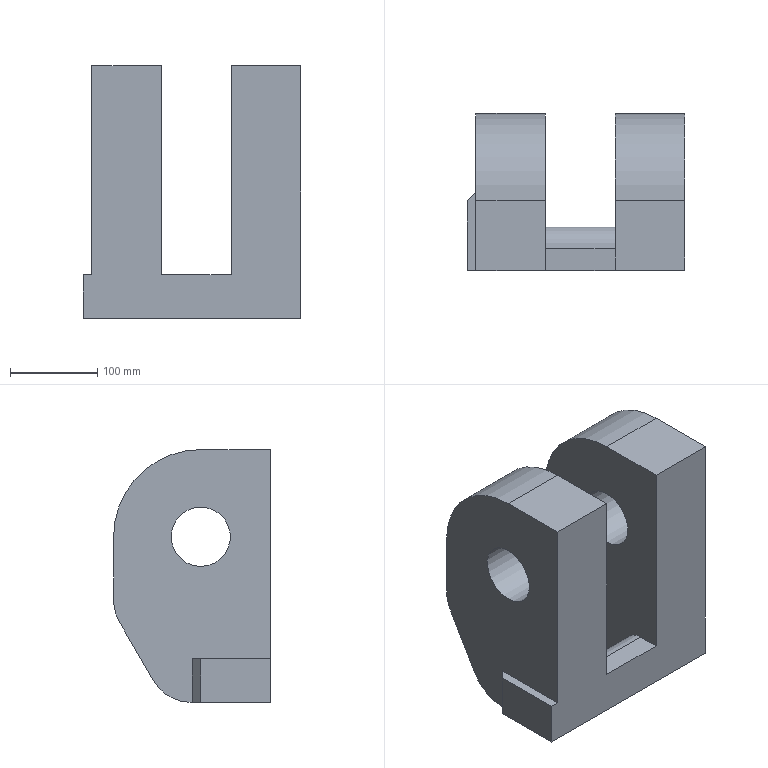Part | NX | features solid 2 | 1 solid | 25 faces | box 250 x 180 x 290 mm | volume 7125817 mm3 | plane 16 | cylinder 9 | commonest cylinder face diameters 100 x4 68 x2 200 x2 50 x1
STEP:
#1=CARTESIAN_POINT('',(-1345.,815.,-350.));
#2=VERTEX_POINT('',#1);
#3=CARTESIAN_POINT('',(-1425.,815.,-350.));
#4=VERTEX_POINT('',#3);
#5=CARTESIAN_POINT('',(-1345.,815.,-350.));
#6=DIRECTION('',(-1.,0.,0.));
#7=VECTOR('',#6,1000.);
#8=LINE('',#5,#7);
#9=EDGE_CURVE('',#2,#4,#8,.T.);
#10=ORIENTED_EDGE('',*,*,#9,.T.);
#11=CARTESIAN_POINT('',(-1425.,715.,-250.));
#12=VERTEX_POINT('',#11);
#13=CARTESIAN_POINT('',(-1425.,715.,-350.));
#14=DIRECTION('',(-1.,0.,0.));
#15=DIRECTION('',(0.,0.,-1.));
#16=AXIS2_PLACEMENT_3D('',#13,#14,#15);
#17=CIRCLE('',#16,100.);
#18=EDGE_CURVE('',#12,#4,#17,.T.);
#19=ORIENTED_EDGE('',*,*,#18,.F.);
#20=CARTESIAN_POINT('',(-1345.,715.,-250.));
#21=VERTEX_POINT('',#20);
#22=CARTESIAN_POINT('',(415.,715.,-250.));
#23=DIRECTION('',(1.,0.,0.));
#24=VECTOR('',#23,1000.);
#25=LINE('',#22,#24);
#26=EDGE_CURVE('',#21,#12,#25,.F.);
#27=ORIENTED_EDGE('',*,*,#26,.F.);
#28=CARTESIAN_POINT('',(-1345.,715.,-350.));
#29=DIRECTION('',(1.,0.,0.));
#30=DIRECTION('',(0.,0.,1.));
#31=AXIS2_PLACEMENT_3D('',#28,#29,#30);
#32=CIRCLE('',#31,100.);
#33=EDGE_CURVE('',#21,#2,#32,.F.);
#34=ORIENTED_EDGE('',*,*,#33,.T.);
#35=EDGE_LOOP('',(#10,#19,#27,#34));
#36=FACE_BOUND('',#35,.T.);
#37=CARTESIAN_POINT('',(415.,715.,-350.));
#38=DIRECTION('',(-1.,0.,0.));
#39=DIRECTION('',(0.,0.,1.));
#40=AXIS2_PLACEMENT_3D('',#37,#38,#39);
#41=CYLINDRICAL_SURFACE('',#40,100.);
#42=ADVANCED_FACE('',(#36),#41,.T.);
#43=CARTESIAN_POINT('',(-1505.,815.,-350.));
#44=VERTEX_POINT('',#43);
#45=CARTESIAN_POINT('',(-1585.,815.,-350.));
#46=VERTEX_POINT('',#45);
#47=CARTESIAN_POINT('',(-1505.,815.,-350.));
#48=DIRECTION('',(-1.,0.,0.));
#49=VECTOR('',#48,1000.);
#50=LINE('',#47,#49);
#51=EDGE_CURVE('',#44,#46,#50,.T.);
#52=ORIENTED_EDGE('',*,*,#51,.T.);
#53=CARTESIAN_POINT('',(-1585.,715.,-250.));
#54=VERTEX_POINT('',#53);
#55=CARTESIAN_POINT('',(-1585.,715.,-350.));
#56=DIRECTION('',(-1.,0.,0.));
#57=DIRECTION('',(0.,0.,-1.));
#58=AXIS2_PLACEMENT_3D('',#55,#56,#57);
#59=CIRCLE('',#58,100.);
#60=EDGE_CURVE('',#54,#46,#59,.T.);
#61=ORIENTED_EDGE('',*,*,#60,.F.);
#62=CARTESIAN_POINT('',(-1505.,715.,-250.));
#63=VERTEX_POINT('',#62);
#64=CARTESIAN_POINT('',(415.,715.,-250.));
#65=DIRECTION('',(1.,0.,0.));
#66=VECTOR('',#65,1000.);
#67=LINE('',#64,#66);
#68=EDGE_CURVE('',#63,#54,#67,.F.);
#69=ORIENTED_EDGE('',*,*,#68,.F.);
#70=CARTESIAN_POINT('',(-1505.,715.,-350.));
#71=DIRECTION('',(1.,0.,0.));
#72=DIRECTION('',(0.,0.,1.));
#73=AXIS2_PLACEMENT_3D('',#70,#71,#72);
#74=CIRCLE('',#73,100.);
#75=EDGE_CURVE('',#63,#44,#74,.F.);
#76=ORIENTED_EDGE('',*,*,#75,.T.);
#77=EDGE_LOOP('',(#52,#61,#69,#76));
#78=FACE_BOUND('',#77,.T.);
#79=CARTESIAN_POINT('',(415.,715.,-350.));
#80=DIRECTION('',(-1.,0.,0.));
#81=DIRECTION('',(0.,0.,1.));
#82=AXIS2_PLACEMENT_3D('',#79,#80,#81);
#83=CYLINDRICAL_SURFACE('',#82,100.);
#84=ADVANCED_FACE('',(#78),#83,.T.);
#85=CARTESIAN_POINT('',(-1345.,635.,-540.));
#86=VERTEX_POINT('',#85);
#87=CARTESIAN_POINT('',(-1345.,635.,-250.));
#88=VERTEX_POINT('',#87);
#89=CARTESIAN_POINT('',(-1345.,635.,-265.));
#90=DIRECTION('',(0.,0.,1.));
#91=VECTOR('',#90,1000.);
#92=LINE('',#89,#91);
#93=EDGE_CURVE('',#86,#88,#92,.T.);
#94=ORIENTED_EDGE('',*,*,#93,.T.);
#95=CARTESIAN_POINT('',(-1425.,635.,-250.));
#96=VERTEX_POINT('',#95);
#97=CARTESIAN_POINT('',(377.,635.,-250.));
#98=DIRECTION('',(-1.,0.,0.));
#99=VECTOR('',#98,1000.);
#100=LINE('',#97,#99);
#101=EDGE_CURVE('',#88,#96,#100,.T.);
#102=ORIENTED_EDGE('',*,*,#101,.T.);
#103=CARTESIAN_POINT('',(-1425.,635.,-490.));
#104=VERTEX_POINT('',#103);
#105=CARTESIAN_POINT('',(-1425.,635.,-350.));
#106=DIRECTION('',(0.,0.,1.));
#107=VECTOR('',#106,1000.);
#108=LINE('',#105,#107);
#109=EDGE_CURVE('',#104,#96,#108,.T.);
#110=ORIENTED_EDGE('',*,*,#109,.F.);
#111=CARTESIAN_POINT('',(-1505.,635.,-490.));
#112=VERTEX_POINT('',#111);
#113=CARTESIAN_POINT('',(1195.,635.,-490.));
#114=DIRECTION('',(-1.,0.,0.));
#115=VECTOR('',#114,1000.);
#116=LINE('',#113,#115);
#117=EDGE_CURVE('',#104,#112,#116,.T.);
#118=ORIENTED_EDGE('',*,*,#117,.T.);
#119=CARTESIAN_POINT('',(-1505.,635.,-250.));
#120=VERTEX_POINT('',#119);
#121=CARTESIAN_POINT('',(-1505.,635.,-265.));
#122=DIRECTION('',(0.,0.,1.));
#123=VECTOR('',#122,1000.);
#124=LINE('',#121,#123);
#125=EDGE_CURVE('',#112,#120,#124,.T.);
#126=ORIENTED_EDGE('',*,*,#125,.T.);
#127=CARTESIAN_POINT('',(-1585.,635.,-250.));
#128=VERTEX_POINT('',#127);
#129=CARTESIAN_POINT('',(377.,635.,-250.));
#130=DIRECTION('',(-1.,0.,0.));
#131=VECTOR('',#130,1000.);
#132=LINE('',#129,#131);
#133=EDGE_CURVE('',#120,#128,#132,.T.);
#134=ORIENTED_EDGE('',*,*,#133,.T.);
#135=CARTESIAN_POINT('',(-1585.,635.,-490.));
#136=VERTEX_POINT('',#135);
#137=CARTESIAN_POINT('',(-1585.,635.,-350.));
#138=DIRECTION('',(0.,0.,1.));
#139=VECTOR('',#138,1000.);
#140=LINE('',#137,#139);
#141=EDGE_CURVE('',#136,#128,#140,.T.);
#142=ORIENTED_EDGE('',*,*,#141,.F.);
#143=CARTESIAN_POINT('',(-1595.,635.,-490.));
#144=VERTEX_POINT('',#143);
#145=CARTESIAN_POINT('',(-1605.,635.,-490.));
#146=DIRECTION('',(1.,0.,0.));
#147=VECTOR('',#146,1000.);
#148=LINE('',#145,#147);
#149=EDGE_CURVE('',#144,#136,#148,.T.);
#150=ORIENTED_EDGE('',*,*,#149,.F.);
#151=CARTESIAN_POINT('',(-1595.,635.,-540.));
#152=VERTEX_POINT('',#151);
#153=CARTESIAN_POINT('',(-1595.,635.,-330.));
#154=DIRECTION('',(0.,0.,1.));
#155=VECTOR('',#154,1000.);
#156=LINE('',#153,#155);
#157=EDGE_CURVE('',#152,#144,#156,.T.);
#158=ORIENTED_EDGE('',*,*,#157,.F.);
#159=CARTESIAN_POINT('',(377.,635.,-540.));
#160=DIRECTION('',(-1.,0.,0.));
#161=VECTOR('',#160,1000.);
#162=LINE('',#159,#161);
#163=EDGE_CURVE('',#86,#152,#162,.T.);
#164=ORIENTED_EDGE('',*,*,#163,.F.);
#165=EDGE_LOOP('',(#94,#102,#110,#118,#126,#134,#142,#150,#158,#164));
#166=FACE_BOUND('',#165,.T.);
#167=CARTESIAN_POINT('',(1195.,635.,-265.));
#168=DIRECTION('',(0.,-1.,0.));
#169=DIRECTION('',(0.,0.,1.));
#170=AXIS2_PLACEMENT_3D('',#167,#168,#169);
#171=PLANE('',#170);
#172=ADVANCED_FACE('',(#166),#171,.T.);
#173=CARTESIAN_POINT('',(-1345.,715.,-316.));
#174=VERTEX_POINT('',#173);
#175=CARTESIAN_POINT('',(-1345.,715.,-350.));
#176=DIRECTION('',(1.,0.,0.));
#177=DIRECTION('',(0.,0.,1.));
#178=AXIS2_PLACEMENT_3D('',#175,#176,#177);
#179=CIRCLE('',#178,34.);
#180=EDGE_CURVE('',#174,#174,#179,.F.);
#181=ORIENTED_EDGE('',*,*,#180,.F.);
#182=EDGE_LOOP('',(#181));
#183=FACE_BOUND('',#182,.T.);
#184=CARTESIAN_POINT('',(-1425.,715.,-384.));
#185=VERTEX_POINT('',#184);
#186=CARTESIAN_POINT('',(-1425.,715.,-350.));
#187=DIRECTION('',(-1.,0.,0.));
#188=DIRECTION('',(0.,0.,-1.));
#189=AXIS2_PLACEMENT_3D('',#186,#187,#188);
#190=CIRCLE('',#189,34.);
#191=EDGE_CURVE('',#185,#185,#190,.F.);
#192=ORIENTED_EDGE('',*,*,#191,.F.);
#193=EDGE_LOOP('',(#192));
#194=FACE_BOUND('',#193,.T.);
#195=CARTESIAN_POINT('',(-1375.,715.,-350.));
#196=DIRECTION('',(-1.,0.,0.));
#197=DIRECTION('',(0.,1.,0.));
#198=AXIS2_PLACEMENT_3D('',#195,#196,#197);
#199=CYLINDRICAL_SURFACE('',#198,34.);
#200=ADVANCED_FACE('',(#183,#194),#199,.F.);
#201=CARTESIAN_POINT('',(-1505.,660.,-490.));
#202=VERTEX_POINT('',#201);
#203=CARTESIAN_POINT('',(-1505.,660.,-540.));
#204=VERTEX_POINT('',#203);
#205=CARTESIAN_POINT('',(-1505.,660.,-515.));
#206=DIRECTION('',(1.,0.,0.));
#207=DIRECTION('',(0.,0.,1.));
#208=AXIS2_PLACEMENT_3D('',#205,#206,#207);
#209=CIRCLE('',#208,25.);
#210=EDGE_CURVE('',#202,#204,#209,.F.);
#211=ORIENTED_EDGE('',*,*,#210,.F.);
#212=CARTESIAN_POINT('',(-1425.,660.,-490.));
#213=VERTEX_POINT('',#212);
#214=CARTESIAN_POINT('',(-1445.,660.,-490.));
#215=DIRECTION('',(-1.,0.,0.));
#216=VECTOR('',#215,1000.);
#217=LINE('',#214,#216);
#218=EDGE_CURVE('',#213,#202,#217,.T.);
#219=ORIENTED_EDGE('',*,*,#218,.F.);
#220=CARTESIAN_POINT('',(-1425.,660.,-540.));
#221=VERTEX_POINT('',#220);
#222=CARTESIAN_POINT('',(-1425.,660.,-515.));
#223=DIRECTION('',(-1.,0.,0.));
#224=DIRECTION('',(0.,1.,0.));
#225=AXIS2_PLACEMENT_3D('',#222,#223,#224);
#226=CIRCLE('',#225,25.);
#227=EDGE_CURVE('',#213,#221,#226,.T.);
#228=ORIENTED_EDGE('',*,*,#227,.T.);
#229=CARTESIAN_POINT('',(-1445.,660.,-540.));
#230=DIRECTION('',(-1.,0.,0.));
#231=VECTOR('',#230,1000.);
#232=LINE('',#229,#231);
#233=EDGE_CURVE('',#221,#204,#232,.T.);
#234=ORIENTED_EDGE('',*,*,#233,.T.);
#235=EDGE_LOOP('',(#211,#219,#228,#234));
#236=FACE_BOUND('',#235,.T.);
#237=CARTESIAN_POINT('',(-1445.,660.,-515.));
#238=DIRECTION('',(-1.,0.,0.));
#239=DIRECTION('',(0.,1.,0.));
#240=AXIS2_PLACEMENT_3D('',#237,#238,#239);
#241=CYLINDRICAL_SURFACE('',#240,25.);
#242=ADVANCED_FACE('',(#236),#241,.T.);
#243=CARTESIAN_POINT('',(-1505.,715.,-316.));
#244=VERTEX_POINT('',#243);
#245=CARTESIAN_POINT('',(-1505.,715.,-350.));
#246=DIRECTION('',(1.,0.,0.));
#247=DIRECTION('',(0.,0.,1.));
#248=AXIS2_PLACEMENT_3D('',#245,#246,#247);
#249=CIRCLE('',#248,34.);
#250=EDGE_CURVE('',#244,#244,#249,.T.);
#251=ORIENTED_EDGE('',*,*,#250,.T.);
#252=EDGE_LOOP('',(#251));
#253=FACE_BOUND('',#252,.T.);
#254=CARTESIAN_POINT('',(-1585.,715.,-384.));
#255=VERTEX_POINT('',#254);
#256=CARTESIAN_POINT('',(-1585.,715.,-350.));
#257=DIRECTION('',(-1.,0.,0.));
#258=DIRECTION('',(0.,0.,-1.));
#259=AXIS2_PLACEMENT_3D('',#256,#257,#258);
#260=CIRCLE('',#259,34.);
#261=EDGE_CURVE('',#255,#255,#260,.F.);
#262=ORIENTED_EDGE('',*,*,#261,.F.);
#263=EDGE_LOOP('',(#262));
#264=FACE_BOUND('',#263,.T.);
#265=CARTESIAN_POINT('',(-1375.,715.,-350.));
#266=DIRECTION('',(-1.,0.,0.));
#267=DIRECTION('',(0.,1.,0.));
#268=AXIS2_PLACEMENT_3D('',#265,#266,#267);
#269=CYLINDRICAL_SURFACE('',#268,34.);
#270=ADVANCED_FACE('',(#253,#264),#269,.F.);
#271=ORIENTED_EDGE('',*,*,#141,.T.);
#272=CARTESIAN_POINT('',(-1585.,640.,-250.));
#273=DIRECTION('',(0.,1.,0.));
#274=VECTOR('',#273,1000.);
#275=LINE('',#272,#274);
#276=EDGE_CURVE('',#128,#54,#275,.T.);
#277=ORIENTED_EDGE('',*,*,#276,.T.);
#278=ORIENTED_EDGE('',*,*,#60,.T.);
#279=CARTESIAN_POINT('',(-1585.,815.,-422.679));
#280=VERTEX_POINT('',#279);
#281=CARTESIAN_POINT('',(-1585.,815.,-350.));
#282=DIRECTION('',(0.,0.,-1.));
#283=VECTOR('',#282,1000.);
#284=LINE('',#281,#283);
#285=EDGE_CURVE('',#46,#280,#284,.T.);
#286=ORIENTED_EDGE('',*,*,#285,.T.);
#287=CARTESIAN_POINT('',(-1585.,808.301,-447.679));
#288=VERTEX_POINT('',#287);
#289=CARTESIAN_POINT('',(-1585.,765.,-422.679));
#290=DIRECTION('',(-1.,0.,0.));
#291=DIRECTION('',(0.,0.,-1.));
#292=AXIS2_PLACEMENT_3D('',#289,#290,#291);
#293=CIRCLE('',#292,50.);
#294=EDGE_CURVE('',#288,#280,#293,.F.);
#295=ORIENTED_EDGE('',*,*,#294,.F.);
#296=CARTESIAN_POINT('',(-1585.,769.434,-515.));
#297=VERTEX_POINT('',#296);
#298=CARTESIAN_POINT('',(-1585.,796.627,-467.901));
#299=DIRECTION('',(0.,0.5,0.866));
#300=VECTOR('',#299,1000.);
#301=LINE('',#298,#300);
#302=EDGE_CURVE('',#297,#288,#301,.T.);
#303=ORIENTED_EDGE('',*,*,#302,.F.);
#304=CARTESIAN_POINT('',(-1585.,726.132,-540.));
#305=VERTEX_POINT('',#304);
#306=CARTESIAN_POINT('',(-1585.,726.132,-490.));
#307=DIRECTION('',(-1.,0.,0.));
#308=DIRECTION('',(0.,0.,-1.));
#309=AXIS2_PLACEMENT_3D('',#306,#307,#308);
#310=CIRCLE('',#309,50.);
#311=EDGE_CURVE('',#305,#297,#310,.F.);
#312=ORIENTED_EDGE('',*,*,#311,.F.);
#313=CARTESIAN_POINT('',(-1585.,725.,-540.));
#314=VERTEX_POINT('',#313);
#315=CARTESIAN_POINT('',(-1585.,800.,-540.));
#316=DIRECTION('',(0.,1.,0.));
#317=VECTOR('',#316,1000.);
#318=LINE('',#315,#317);
#319=EDGE_CURVE('',#314,#305,#318,.T.);
#320=ORIENTED_EDGE('',*,*,#319,.F.);
#321=CARTESIAN_POINT('',(-1585.,725.,-490.));
#322=VERTEX_POINT('',#321);
#323=CARTESIAN_POINT('',(-1585.,725.,-540.));
#324=DIRECTION('',(0.,0.,1.));
#325=VECTOR('',#324,1000.);
#326=LINE('',#323,#325);
#327=EDGE_CURVE('',#314,#322,#326,.T.);
#328=ORIENTED_EDGE('',*,*,#327,.T.);
#329=CARTESIAN_POINT('',(-1585.,680.,-490.));
#330=DIRECTION('',(0.,1.,0.));
#331=VECTOR('',#330,1000.);
#332=LINE('',#329,#331);
#333=EDGE_CURVE('',#136,#322,#332,.T.);
#334=ORIENTED_EDGE('',*,*,#333,.F.);
#335=EDGE_LOOP('',(#271,#277,#278,#286,#295,#303,#312,#320,#328,#334));
#336=FACE_BOUND('',#335,.T.);
#337=ORIENTED_EDGE('',*,*,#261,.T.);
#338=EDGE_LOOP('',(#337));
#339=FACE_BOUND('',#338,.T.);
#340=CARTESIAN_POINT('',(-1585.,715.,-350.));
#341=DIRECTION('',(1.,0.,0.));
#342=DIRECTION('',(0.,-1.,0.));
#343=AXIS2_PLACEMENT_3D('',#340,#341,#342);
#344=PLANE('',#343);
#345=ADVANCED_FACE('',(#336,#339),#344,.F.);
#346=CARTESIAN_POINT('',(-1505.,715.,-490.));
#347=DIRECTION('',(0.,1.,0.));
#348=VECTOR('',#347,1000.);
#349=LINE('',#346,#348);
#350=EDGE_CURVE('',#112,#202,#349,.T.);
#351=ORIENTED_EDGE('',*,*,#350,.F.);
#352=ORIENTED_EDGE('',*,*,#117,.F.);
#353=CARTESIAN_POINT('',(-1425.,640.,-490.));
#354=DIRECTION('',(0.,1.,0.));
#355=VECTOR('',#354,1000.);
#356=LINE('',#353,#355);
#357=EDGE_CURVE('',#104,#213,#356,.T.);
#358=ORIENTED_EDGE('',*,*,#357,.T.);
#359=ORIENTED_EDGE('',*,*,#218,.T.);
#360=EDGE_LOOP('',(#351,#352,#358,#359));
#361=FACE_BOUND('',#360,.T.);
#362=CARTESIAN_POINT('',(-1445.,640.,-490.));
#363=DIRECTION('',(0.,0.,-1.));
#364=DIRECTION('',(0.,-1.,0.));
#365=AXIS2_PLACEMENT_3D('',#362,#363,#364);
#366=PLANE('',#365);
#367=ADVANCED_FACE('',(#361),#366,.F.);
#368=CARTESIAN_POINT('',(-1505.,769.434,-515.));
#369=VERTEX_POINT('',#368);
#370=CARTESIAN_POINT('',(-1505.,808.301,-447.679));
#371=VERTEX_POINT('',#370);
#372=CARTESIAN_POINT('',(-1505.,796.627,-467.901));
#373=DIRECTION('',(0.,0.5,0.866));
#374=VECTOR('',#373,1000.);
#375=LINE('',#372,#374);
#376=EDGE_CURVE('',#369,#371,#375,.T.);
#377=ORIENTED_EDGE('',*,*,#376,.T.);
#378=CARTESIAN_POINT('',(-1505.,815.,-422.679));
#379=VERTEX_POINT('',#378);
#380=CARTESIAN_POINT('',(-1505.,765.,-422.679));
#381=DIRECTION('',(-1.,0.,0.));
#382=DIRECTION('',(0.,0.,-1.));
#383=AXIS2_PLACEMENT_3D('',#380,#381,#382);
#384=CIRCLE('',#383,50.);
#385=EDGE_CURVE('',#379,#371,#384,.T.);
#386=ORIENTED_EDGE('',*,*,#385,.F.);
#387=CARTESIAN_POINT('',(-1505.,815.,-350.));
#388=DIRECTION('',(0.,0.,-1.));
#389=VECTOR('',#388,1000.);
#390=LINE('',#387,#389);
#391=EDGE_CURVE('',#44,#379,#390,.T.);
#392=ORIENTED_EDGE('',*,*,#391,.F.);
#393=ORIENTED_EDGE('',*,*,#75,.F.);
#394=CARTESIAN_POINT('',(-1505.,220.,-250.));
#395=DIRECTION('',(0.,1.,0.));
#396=VECTOR('',#395,1000.);
#397=LINE('',#394,#396);
#398=EDGE_CURVE('',#120,#63,#397,.T.);
#399=ORIENTED_EDGE('',*,*,#398,.F.);
#400=ORIENTED_EDGE('',*,*,#125,.F.);
#401=ORIENTED_EDGE('',*,*,#350,.T.);
#402=ORIENTED_EDGE('',*,*,#210,.T.);
#403=CARTESIAN_POINT('',(-1505.,726.132,-540.));
#404=VERTEX_POINT('',#403);
#405=CARTESIAN_POINT('',(-1505.,715.,-540.));
#406=DIRECTION('',(0.,1.,0.));
#407=VECTOR('',#406,1000.);
#408=LINE('',#405,#407);
#409=EDGE_CURVE('',#404,#204,#408,.F.);
#410=ORIENTED_EDGE('',*,*,#409,.F.);
#411=CARTESIAN_POINT('',(-1505.,726.132,-490.));
#412=DIRECTION('',(-1.,0.,0.));
#413=DIRECTION('',(0.,0.,-1.));
#414=AXIS2_PLACEMENT_3D('',#411,#412,#413);
#415=CIRCLE('',#414,50.);
#416=EDGE_CURVE('',#369,#404,#415,.T.);
#417=ORIENTED_EDGE('',*,*,#416,.F.);
#418=EDGE_LOOP('',(#377,#386,#392,#393,#399,#400,#401,#402,#410,#417));
#419=FACE_BOUND('',#418,.T.);
#420=ORIENTED_EDGE('',*,*,#250,.F.);
#421=EDGE_LOOP('',(#420));
#422=FACE_BOUND('',#421,.T.);
#423=CARTESIAN_POINT('',(-1505.,715.,-350.));
#424=DIRECTION('',(1.,0.,0.));
#425=DIRECTION('',(0.,-1.,0.));
#426=AXIS2_PLACEMENT_3D('',#423,#424,#425);
#427=PLANE('',#426);
#428=ADVANCED_FACE('',(#419,#422),#427,.T.);
#429=CARTESIAN_POINT('',(-1425.,726.132,-540.));
#430=VERTEX_POINT('',#429);
#431=CARTESIAN_POINT('',(-1425.,715.,-540.));
#432=DIRECTION('',(0.,1.,0.));
#433=VECTOR('',#432,1000.);
#434=LINE('',#431,#433);
#435=EDGE_CURVE('',#430,#221,#434,.F.);
#436=ORIENTED_EDGE('',*,*,#435,.T.);
#437=ORIENTED_EDGE('',*,*,#227,.F.);
#438=ORIENTED_EDGE('',*,*,#357,.F.);
#439=ORIENTED_EDGE('',*,*,#109,.T.);
#440=CARTESIAN_POINT('',(-1425.,640.,-250.));
#441=DIRECTION('',(0.,1.,0.));
#442=VECTOR('',#441,1000.);
#443=LINE('',#440,#442);
#444=EDGE_CURVE('',#96,#12,#443,.T.);
#445=ORIENTED_EDGE('',*,*,#444,.T.);
#446=ORIENTED_EDGE('',*,*,#18,.T.);
#447=CARTESIAN_POINT('',(-1425.,815.,-422.679));
#448=VERTEX_POINT('',#447);
#449=CARTESIAN_POINT('',(-1425.,815.,-350.));
#450=DIRECTION('',(0.,0.,-1.));
#451=VECTOR('',#450,1000.);
#452=LINE('',#449,#451);
#453=EDGE_CURVE('',#4,#448,#452,.T.);
#454=ORIENTED_EDGE('',*,*,#453,.T.);
#455=CARTESIAN_POINT('',(-1425.,808.301,-447.679));
#456=VERTEX_POINT('',#455);
#457=CARTESIAN_POINT('',(-1425.,765.,-422.679));
#458=DIRECTION('',(-1.,0.,0.));
#459=DIRECTION('',(0.,0.,-1.));
#460=AXIS2_PLACEMENT_3D('',#457,#458,#459);
#461=CIRCLE('',#460,50.);
#462=EDGE_CURVE('',#456,#448,#461,.F.);
#463=ORIENTED_EDGE('',*,*,#462,.F.);
#464=CARTESIAN_POINT('',(-1425.,769.434,-515.));
#465=VERTEX_POINT('',#464);
#466=CARTESIAN_POINT('',(-1425.,796.627,-467.901));
#467=DIRECTION('',(0.,0.5,0.866));
#468=VECTOR('',#467,1000.);
#469=LINE('',#466,#468);
#470=EDGE_CURVE('',#465,#456,#469,.T.);
#471=ORIENTED_EDGE('',*,*,#470,.F.);
#472=CARTESIAN_POINT('',(-1425.,726.132,-490.));
#473=DIRECTION('',(-1.,0.,0.));
#474=DIRECTION('',(0.,0.,-1.));
#475=AXIS2_PLACEMENT_3D('',#472,#473,#474);
#476=CIRCLE('',#475,50.);
#477=EDGE_CURVE('',#430,#465,#476,.F.);
#478=ORIENTED_EDGE('',*,*,#477,.F.);
#479=EDGE_LOOP('',(#436,#437,#438,#439,#445,#446,#454,#463,#471,#478));
#480=FACE_BOUND('',#479,.T.);
#481=ORIENTED_EDGE('',*,*,#191,.T.);
#482=EDGE_LOOP('',(#481));
#483=FACE_BOUND('',#482,.T.);
#484=CARTESIAN_POINT('',(-1425.,715.,-350.));
#485=DIRECTION('',(1.,0.,0.));
#486=DIRECTION('',(0.,-1.,0.));
#487=AXIS2_PLACEMENT_3D('',#484,#485,#486);
#488=PLANE('',#487);
#489=ADVANCED_FACE('',(#480,#483),#488,.F.);
#490=CARTESIAN_POINT('',(-1345.,769.434,-515.));
#491=VERTEX_POINT('',#490);
#492=CARTESIAN_POINT('',(-1345.,808.301,-447.679));
#493=VERTEX_POINT('',#492);
#494=CARTESIAN_POINT('',(-1345.,612.341,-787.092));
#495=DIRECTION('',(0.,0.5,0.866));
#496=VECTOR('',#495,1000.);
#497=LINE('',#494,#496);
#498=EDGE_CURVE('',#491,#493,#497,.T.);
#499=ORIENTED_EDGE('',*,*,#498,.T.);
#500=CARTESIAN_POINT('',(-1345.,815.,-422.679));
#501=VERTEX_POINT('',#500);
#502=CARTESIAN_POINT('',(-1345.,765.,-422.679));
#503=DIRECTION('',(-1.,0.,0.));
#504=DIRECTION('',(0.,0.,-1.));
#505=AXIS2_PLACEMENT_3D('',#502,#503,#504);
#506=CIRCLE('',#505,50.);
#507=EDGE_CURVE('',#501,#493,#506,.T.);
#508=ORIENTED_EDGE('',*,*,#507,.F.);
#509=CARTESIAN_POINT('',(-1345.,815.,-350.));
#510=DIRECTION('',(0.,0.,-1.));
#511=VECTOR('',#510,1000.);
#512=LINE('',#509,#511);
#513=EDGE_CURVE('',#2,#501,#512,.T.);
#514=ORIENTED_EDGE('',*,*,#513,.F.);
#515=ORIENTED_EDGE('',*,*,#33,.F.);
#516=CARTESIAN_POINT('',(-1345.,220.,-250.));
#517=DIRECTION('',(0.,1.,0.));
#518=VECTOR('',#517,1000.);
#519=LINE('',#516,#518);
#520=EDGE_CURVE('',#88,#21,#519,.T.);
#521=ORIENTED_EDGE('',*,*,#520,.F.);
#522=ORIENTED_EDGE('',*,*,#93,.F.);
#523=CARTESIAN_POINT('',(-1345.,726.132,-540.));
#524=VERTEX_POINT('',#523);
#525=CARTESIAN_POINT('',(-1345.,12.5,-540.));
#526=DIRECTION('',(0.,1.,0.));
#527=VECTOR('',#526,1000.);
#528=LINE('',#525,#527);
#529=EDGE_CURVE('',#524,#86,#528,.F.);
#530=ORIENTED_EDGE('',*,*,#529,.F.);
#531=CARTESIAN_POINT('',(-1345.,726.132,-490.));
#532=DIRECTION('',(-1.,0.,0.));
#533=DIRECTION('',(0.,0.,-1.));
#534=AXIS2_PLACEMENT_3D('',#531,#532,#533);
#535=CIRCLE('',#534,50.);
#536=EDGE_CURVE('',#491,#524,#535,.T.);
#537=ORIENTED_EDGE('',*,*,#536,.F.);
#538=EDGE_LOOP('',(#499,#508,#514,#515,#521,#522,#530,#537));
#539=FACE_BOUND('',#538,.T.);
#540=ORIENTED_EDGE('',*,*,#180,.T.);
#541=EDGE_LOOP('',(#540));
#542=FACE_BOUND('',#541,.T.);
#543=CARTESIAN_POINT('',(-1345.,12.5,-370.));
#544=DIRECTION('',(1.,0.,0.));
#545=DIRECTION('',(0.,0.,-1.));
#546=AXIS2_PLACEMENT_3D('',#543,#544,#545);
#547=PLANE('',#546);
#548=ADVANCED_FACE('',(#539,#542),#547,.T.);
#549=ORIENTED_EDGE('',*,*,#398,.T.);
#550=ORIENTED_EDGE('',*,*,#68,.T.);
#551=ORIENTED_EDGE('',*,*,#276,.F.);
#552=ORIENTED_EDGE('',*,*,#133,.F.);
#553=EDGE_LOOP('',(#549,#550,#551,#552));
#554=FACE_BOUND('',#553,.T.);
#555=CARTESIAN_POINT('',(377.,220.,-250.));
#556=DIRECTION('',(0.,0.,1.));
#557=DIRECTION('',(-1.,0.,0.));
#558=AXIS2_PLACEMENT_3D('',#555,#556,#557);
#559=PLANE('',#558);
#560=ADVANCED_FACE('',(#554),#559,.T.);
#561=ORIENTED_EDGE('',*,*,#520,.T.);
#562=ORIENTED_EDGE('',*,*,#26,.T.);
#563=ORIENTED_EDGE('',*,*,#444,.F.);
#564=ORIENTED_EDGE('',*,*,#101,.F.);
#565=EDGE_LOOP('',(#561,#562,#563,#564));
#566=FACE_BOUND('',#565,.T.);
#567=CARTESIAN_POINT('',(377.,220.,-250.));
#568=DIRECTION('',(0.,0.,1.));
#569=DIRECTION('',(-1.,0.,0.));
#570=AXIS2_PLACEMENT_3D('',#567,#568,#569);
#571=PLANE('',#570);
#572=ADVANCED_FACE('',(#566),#571,.T.);
#573=ORIENTED_EDGE('',*,*,#285,.F.);
#574=ORIENTED_EDGE('',*,*,#51,.F.);
#575=ORIENTED_EDGE('',*,*,#391,.T.);
#576=CARTESIAN_POINT('',(-1505.,815.,-422.679));
#577=DIRECTION('',(1.,0.,0.));
#578=VECTOR('',#577,1000.);
#579=LINE('',#576,#578);
#580=EDGE_CURVE('',#280,#379,#579,.T.);
#581=ORIENTED_EDGE('',*,*,#580,.F.);
#582=EDGE_LOOP('',(#573,#574,#575,#581));
#583=FACE_BOUND('',#582,.T.);
#584=CARTESIAN_POINT('',(-1505.,815.,-350.));
#585=DIRECTION('',(0.,-1.,0.));
#586=DIRECTION('',(0.,0.,1.));
#587=AXIS2_PLACEMENT_3D('',#584,#585,#586);
#588=PLANE('',#587);
#589=ADVANCED_FACE('',(#583),#588,.F.);
#590=ORIENTED_EDGE('',*,*,#409,.T.);
#591=ORIENTED_EDGE('',*,*,#233,.F.);
#592=ORIENTED_EDGE('',*,*,#435,.F.);
#593=CARTESIAN_POINT('',(-1345.,726.132,-540.));
#594=DIRECTION('',(-1.,0.,0.));
#595=VECTOR('',#594,1000.);
#596=LINE('',#593,#595);
#597=EDGE_CURVE('',#524,#430,#596,.T.);
#598=ORIENTED_EDGE('',*,*,#597,.F.);
#599=ORIENTED_EDGE('',*,*,#529,.T.);
#600=ORIENTED_EDGE('',*,*,#163,.T.);
#601=CARTESIAN_POINT('',(-1595.,715.,-540.));
#602=VERTEX_POINT('',#601);
#603=CARTESIAN_POINT('',(-1595.,815.,-540.));
#604=DIRECTION('',(0.,-1.,0.));
#605=VECTOR('',#604,1000.);
#606=LINE('',#603,#605);
#607=EDGE_CURVE('',#152,#602,#606,.F.);
#608=ORIENTED_EDGE('',*,*,#607,.T.);
#609=CARTESIAN_POINT('',(-1617.5,692.5,-540.));
#610=DIRECTION('',(0.7071,0.7071,0.));
#611=VECTOR('',#610,1000.);
#612=LINE('',#609,#611);
#613=EDGE_CURVE('',#314,#602,#612,.F.);
#614=ORIENTED_EDGE('',*,*,#613,.F.);
#615=ORIENTED_EDGE('',*,*,#319,.T.);
#616=CARTESIAN_POINT('',(-1345.,726.132,-540.));
#617=DIRECTION('',(-1.,0.,0.));
#618=VECTOR('',#617,1000.);
#619=LINE('',#616,#618);
#620=EDGE_CURVE('',#404,#305,#619,.T.);
#621=ORIENTED_EDGE('',*,*,#620,.F.);
#622=EDGE_LOOP('',(#590,#591,#592,#598,#599,#600,#608,#614,#615,#621));
#623=FACE_BOUND('',#622,.T.);
#624=CARTESIAN_POINT('',(-1345.,815.,-540.));
#625=DIRECTION('',(0.,0.,-1.));
#626=DIRECTION('',(-1.,0.,0.));
#627=AXIS2_PLACEMENT_3D('',#624,#625,#626);
#628=PLANE('',#627);
#629=ADVANCED_FACE('',(#623),#628,.T.);
#630=ORIENTED_EDGE('',*,*,#453,.F.);
#631=ORIENTED_EDGE('',*,*,#9,.F.);
#632=ORIENTED_EDGE('',*,*,#513,.T.);
#633=CARTESIAN_POINT('',(-1345.,815.,-422.679));
#634=DIRECTION('',(1.,0.,0.));
#635=VECTOR('',#634,1000.);
#636=LINE('',#633,#635);
#637=EDGE_CURVE('',#448,#501,#636,.T.);
#638=ORIENTED_EDGE('',*,*,#637,.F.);
#639=EDGE_LOOP('',(#630,#631,#632,#638));
#640=FACE_BOUND('',#639,.T.);
#641=CARTESIAN_POINT('',(-1345.,815.,-350.));
#642=DIRECTION('',(0.,-1.,0.));
#643=DIRECTION('',(0.,0.,1.));
#644=AXIS2_PLACEMENT_3D('',#641,#642,#643);
#645=PLANE('',#644);
#646=ADVANCED_FACE('',(#640),#645,.F.);
#647=ORIENTED_EDGE('',*,*,#470,.T.);
#648=CARTESIAN_POINT('',(-1585.,808.301,-447.679));
#649=DIRECTION('',(1.,0.,0.));
#650=VECTOR('',#649,1000.);
#651=LINE('',#648,#650);
#652=EDGE_CURVE('',#493,#456,#651,.F.);
#653=ORIENTED_EDGE('',*,*,#652,.F.);
#654=ORIENTED_EDGE('',*,*,#498,.F.);
#655=CARTESIAN_POINT('',(-1585.,769.434,-515.));
#656=DIRECTION('',(1.,0.,0.));
#657=VECTOR('',#656,1000.);
#658=LINE('',#655,#657);
#659=EDGE_CURVE('',#465,#491,#658,.T.);
#660=ORIENTED_EDGE('',*,*,#659,.F.);
#661=EDGE_LOOP('',(#647,#653,#654,#660));
#662=FACE_BOUND('',#661,.T.);
#663=CARTESIAN_POINT('',(-1585.,755.,-540.));
#664=DIRECTION('',(0.,-0.866,0.5));
#665=DIRECTION('',(0.,0.5,0.866));
#666=AXIS2_PLACEMENT_3D('',#663,#664,#665);
#667=PLANE('',#666);
#668=ADVANCED_FACE('',(#662),#667,.F.);
#669=ORIENTED_EDGE('',*,*,#302,.T.);
#670=CARTESIAN_POINT('',(-1585.,808.301,-447.679));
#671=DIRECTION('',(1.,0.,0.));
#672=VECTOR('',#671,1000.);
#673=LINE('',#670,#672);
#674=EDGE_CURVE('',#371,#288,#673,.F.);
#675=ORIENTED_EDGE('',*,*,#674,.F.);
#676=ORIENTED_EDGE('',*,*,#376,.F.);
#677=CARTESIAN_POINT('',(-1585.,769.434,-515.));
#678=DIRECTION('',(1.,0.,0.));
#679=VECTOR('',#678,1000.);
#680=LINE('',#677,#679);
#681=EDGE_CURVE('',#297,#369,#680,.T.);
#682=ORIENTED_EDGE('',*,*,#681,.F.);
#683=EDGE_LOOP('',(#669,#675,#676,#682));
#684=FACE_BOUND('',#683,.T.);
#685=CARTESIAN_POINT('',(-1585.,755.,-540.));
#686=DIRECTION('',(0.,-0.866,0.5));
#687=DIRECTION('',(0.,0.5,0.866));
#688=AXIS2_PLACEMENT_3D('',#685,#686,#687);
#689=PLANE('',#688);
#690=ADVANCED_FACE('',(#684),#689,.F.);
#691=ORIENTED_EDGE('',*,*,#416,.T.);
#692=ORIENTED_EDGE('',*,*,#620,.T.);
#693=ORIENTED_EDGE('',*,*,#311,.T.);
#694=ORIENTED_EDGE('',*,*,#681,.T.);
#695=EDGE_LOOP('',(#691,#692,#693,#694));
#696=FACE_BOUND('',#695,.T.);
#697=CARTESIAN_POINT('',(-1345.,726.132,-490.));
#698=DIRECTION('',(1.,0.,0.));
#699=DIRECTION('',(0.,-1.,0.));
#700=AXIS2_PLACEMENT_3D('',#697,#698,#699);
#701=CYLINDRICAL_SURFACE('',#700,50.);
#702=ADVANCED_FACE('',(#696),#701,.T.);
#703=ORIENTED_EDGE('',*,*,#536,.T.);
#704=ORIENTED_EDGE('',*,*,#597,.T.);
#705=ORIENTED_EDGE('',*,*,#477,.T.);
#706=ORIENTED_EDGE('',*,*,#659,.T.);
#707=EDGE_LOOP('',(#703,#704,#705,#706));
#708=FACE_BOUND('',#707,.T.);
#709=CARTESIAN_POINT('',(-1345.,726.132,-490.));
#710=DIRECTION('',(1.,0.,0.));
#711=DIRECTION('',(0.,-1.,0.));
#712=AXIS2_PLACEMENT_3D('',#709,#710,#711);
#713=CYLINDRICAL_SURFACE('',#712,50.);
#714=ADVANCED_FACE('',(#708),#713,.T.);
#715=ORIENTED_EDGE('',*,*,#462,.T.);
#716=ORIENTED_EDGE('',*,*,#637,.T.);
#717=ORIENTED_EDGE('',*,*,#507,.T.);
#718=ORIENTED_EDGE('',*,*,#652,.T.);
#719=EDGE_LOOP('',(#715,#716,#717,#718));
#720=FACE_BOUND('',#719,.T.);
#721=CARTESIAN_POINT('',(-1345.,765.,-422.679));
#722=DIRECTION('',(1.,0.,0.));
#723=DIRECTION('',(0.,0.,-1.));
#724=AXIS2_PLACEMENT_3D('',#721,#722,#723);
#725=CYLINDRICAL_SURFACE('',#724,50.);
#726=ADVANCED_FACE('',(#720),#725,.T.);
#727=ORIENTED_EDGE('',*,*,#294,.T.);
#728=ORIENTED_EDGE('',*,*,#580,.T.);
#729=ORIENTED_EDGE('',*,*,#385,.T.);
#730=ORIENTED_EDGE('',*,*,#674,.T.);
#731=EDGE_LOOP('',(#727,#728,#729,#730));
#732=FACE_BOUND('',#731,.T.);
#733=CARTESIAN_POINT('',(-1505.,765.,-422.679));
#734=DIRECTION('',(1.,0.,0.));
#735=DIRECTION('',(0.,0.,-1.));
#736=AXIS2_PLACEMENT_3D('',#733,#734,#735);
#737=CYLINDRICAL_SURFACE('',#736,50.);
#738=ADVANCED_FACE('',(#732),#737,.T.);
#739=CARTESIAN_POINT('',(-1595.,715.,-490.));
#740=VERTEX_POINT('',#739);
#741=CARTESIAN_POINT('',(-1595.,-845.,-490.));
#742=DIRECTION('',(0.,-1.,0.));
#743=VECTOR('',#742,1000.);
#744=LINE('',#741,#743);
#745=EDGE_CURVE('',#740,#144,#744,.T.);
#746=ORIENTED_EDGE('',*,*,#745,.T.);
#747=ORIENTED_EDGE('',*,*,#149,.T.);
#748=ORIENTED_EDGE('',*,*,#333,.T.);
#749=CARTESIAN_POINT('',(-1617.5,692.5,-490.));
#750=DIRECTION('',(-0.7071,-0.7071,0.));
#751=VECTOR('',#750,1000.);
#752=LINE('',#749,#751);
#753=EDGE_CURVE('',#740,#322,#752,.F.);
#754=ORIENTED_EDGE('',*,*,#753,.F.);
#755=EDGE_LOOP('',(#746,#747,#748,#754));
#756=FACE_BOUND('',#755,.T.);
#757=CARTESIAN_POINT('',(-1605.,680.,-490.));
#758=DIRECTION('',(0.,0.,1.));
#759=DIRECTION('',(1.,0.,0.));
#760=AXIS2_PLACEMENT_3D('',#757,#758,#759);
#761=PLANE('',#760);
#762=ADVANCED_FACE('',(#756),#761,.T.);
#763=ORIENTED_EDGE('',*,*,#607,.F.);
#764=ORIENTED_EDGE('',*,*,#157,.T.);
#765=ORIENTED_EDGE('',*,*,#745,.F.);
#766=CARTESIAN_POINT('',(-1595.,715.,-65.));
#767=DIRECTION('',(0.,0.,-1.));
#768=VECTOR('',#767,1000.);
#769=LINE('',#766,#768);
#770=EDGE_CURVE('',#602,#740,#769,.F.);
#771=ORIENTED_EDGE('',*,*,#770,.F.);
#772=EDGE_LOOP('',(#763,#764,#765,#771));
#773=FACE_BOUND('',#772,.T.);
#774=CARTESIAN_POINT('',(-1595.,-845.,-65.));
#775=DIRECTION('',(-1.,0.,0.));
#776=DIRECTION('',(0.,-1.,0.));
#777=AXIS2_PLACEMENT_3D('',#774,#775,#776);
#778=PLANE('',#777);
#779=ADVANCED_FACE('',(#773),#778,.T.);
#780=ORIENTED_EDGE('',*,*,#613,.T.);
#781=ORIENTED_EDGE('',*,*,#770,.T.);
#782=ORIENTED_EDGE('',*,*,#753,.T.);
#783=ORIENTED_EDGE('',*,*,#327,.F.);
#784=EDGE_LOOP('',(#780,#781,#782,#783));
#785=FACE_BOUND('',#784,.T.);
#786=CARTESIAN_POINT('',(-1625.,685.,-540.));
#787=DIRECTION('',(0.7071,-0.7071,0.));
#788=DIRECTION('',(-0.7071,-0.7071,0.));
#789=AXIS2_PLACEMENT_3D('',#786,#787,#788);
#790=PLANE('',#789);
#791=ADVANCED_FACE('',(#785),#790,.F.);
#792=CLOSED_SHELL('',(#42,#84,#172,#200,#242,#270,#345,#367,#428,#489,#548,#560,#572,#589,#629,#646,#668,#690,#702,#714,#726,#738,#762,#779,#791));
#793=MANIFOLD_SOLID_BREP('',#792);
#794=(LENGTH_UNIT()NAMED_UNIT(*)SI_UNIT(.MILLI.,.METRE.));
#795=UNCERTAINTY_MEASURE_WITH_UNIT(LENGTH_MEASURE(0.00001),#794,'','');
#796=(NAMED_UNIT(*)PLANE_ANGLE_UNIT()SI_UNIT($,.RADIAN.));
#797=(NAMED_UNIT(*)SI_UNIT($,.STERADIAN.)SOLID_ANGLE_UNIT());
#798=(GEOMETRIC_REPRESENTATION_CONTEXT(3)GLOBAL_UNCERTAINTY_ASSIGNED_CONTEXT((#795))GLOBAL_UNIT_ASSIGNED_CONTEXT((#794,#796,#797))REPRESENTATION_CONTEXT('',''));
#799=ADVANCED_BREP_SHAPE_REPRESENTATION('',(#793),#798);